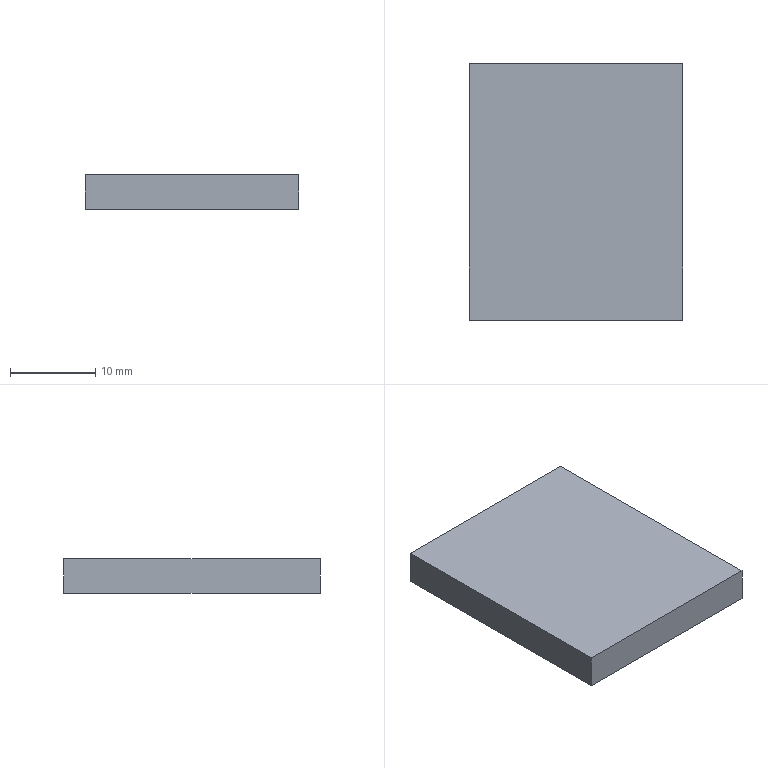Part | STEP file | Q7C0516 | 1 solid | 6 faces | box 25 x 30 x 4 mm | volume 3000 mm3 | plane 6
STEP:
#1=CARTESIAN_POINT('',(0.,0.,0.));
#2=DIRECTION('',(0.,0.,1.));
#3=DIRECTION('',(1.,0.,0.));
#4=AXIS2_PLACEMENT_3D('',#1,#2,#3);
#5=CARTESIAN_POINT('',(-25.,0.,0.));
#6=VERTEX_POINT('',#5);
#7=CARTESIAN_POINT('',(0.,0.,0.));
#8=VERTEX_POINT('',#7);
#9=CARTESIAN_POINT('',(-25.,0.,0.));
#10=DIRECTION('',(1.,0.,0.));
#11=VECTOR('',#10,1.);
#12=LINE('',#9,#11);
#13=CARTESIAN_POINT('',(-25.,0.,4.));
#14=DIRECTION('',(0.,1.,0.));
#15=DIRECTION('',(0.,0.,1.));
#16=AXIS2_PLACEMENT_3D('',#13,#14,#15);
#17=PLANE('',#16);
#18=CARTESIAN_POINT('',(-4.,0.));
#19=DIRECTION('',(0.,1.));
#20=VECTOR('',#19,1.);
#21=LINE('',#18,#20);
#22=(GEOMETRIC_REPRESENTATION_CONTEXT(2)PARAMETRIC_REPRESENTATION_CONTEXT()REPRESENTATION_CONTEXT('',''));
#23=DEFINITIONAL_REPRESENTATION('',(#21),#22);
#24=PCURVE('',#17,#23);
#25=CARTESIAN_POINT('',(0.,0.,0.));
#26=DIRECTION('',(0.,0.,1.));
#27=DIRECTION('',(1.,0.,0.));
#28=AXIS2_PLACEMENT_3D('',#25,#26,#27);
#29=PLANE('',#28);
#30=CARTESIAN_POINT('',(-25.,0.));
#31=DIRECTION('',(1.,0.));
#32=VECTOR('',#31,1.);
#33=LINE('',#30,#32);
#34=(GEOMETRIC_REPRESENTATION_CONTEXT(2)PARAMETRIC_REPRESENTATION_CONTEXT()REPRESENTATION_CONTEXT('',''));
#35=DEFINITIONAL_REPRESENTATION('',(#33),#34);
#36=PCURVE('',#29,#35);
#37=SURFACE_CURVE('',#12,(#24,#36),.PCURVE_S1.);
#38=EDGE_CURVE('',#6,#8,#37,.T.);
#39=ORIENTED_EDGE('',*,*,#38,.T.);
#40=CARTESIAN_POINT('',(0.,0.,4.));
#41=VERTEX_POINT('',#40);
#42=CARTESIAN_POINT('',(0.,0.,4.));
#43=DIRECTION('',(0.,0.,-1.));
#44=VECTOR('',#43,1.);
#45=LINE('',#42,#44);
#46=CARTESIAN_POINT('',(0.,25.));
#47=DIRECTION('',(-1.,0.));
#48=VECTOR('',#47,1.);
#49=LINE('',#46,#48);
#50=(GEOMETRIC_REPRESENTATION_CONTEXT(2)PARAMETRIC_REPRESENTATION_CONTEXT()REPRESENTATION_CONTEXT('',''));
#51=DEFINITIONAL_REPRESENTATION('',(#49),#50);
#52=PCURVE('',#17,#51);
#53=CARTESIAN_POINT('',(0.,0.,4.));
#54=DIRECTION('',(-1.,0.,0.));
#55=DIRECTION('',(0.,0.,1.));
#56=AXIS2_PLACEMENT_3D('',#53,#54,#55);
#57=PLANE('',#56);
#58=CARTESIAN_POINT('',(0.,0.));
#59=DIRECTION('',(-1.,0.));
#60=VECTOR('',#59,1.);
#61=LINE('',#58,#60);
#62=(GEOMETRIC_REPRESENTATION_CONTEXT(2)PARAMETRIC_REPRESENTATION_CONTEXT()REPRESENTATION_CONTEXT('',''));
#63=DEFINITIONAL_REPRESENTATION('',(#61),#62);
#64=PCURVE('',#57,#63);
#65=SURFACE_CURVE('',#45,(#52,#64),.PCURVE_S1.);
#66=EDGE_CURVE('',#41,#8,#65,.T.);
#67=ORIENTED_EDGE('',*,*,#66,.F.);
#68=CARTESIAN_POINT('',(-25.,0.,4.));
#69=VERTEX_POINT('',#68);
#70=CARTESIAN_POINT('',(-25.,0.,4.));
#71=DIRECTION('',(1.,0.,0.));
#72=VECTOR('',#71,1.);
#73=LINE('',#70,#72);
#74=CARTESIAN_POINT('',(0.,0.));
#75=DIRECTION('',(0.,1.));
#76=VECTOR('',#75,1.);
#77=LINE('',#74,#76);
#78=(GEOMETRIC_REPRESENTATION_CONTEXT(2)PARAMETRIC_REPRESENTATION_CONTEXT()REPRESENTATION_CONTEXT('',''));
#79=DEFINITIONAL_REPRESENTATION('',(#77),#78);
#80=PCURVE('',#17,#79);
#81=CARTESIAN_POINT('',(0.,0.,4.));
#82=DIRECTION('',(0.,0.,1.));
#83=DIRECTION('',(1.,0.,0.));
#84=AXIS2_PLACEMENT_3D('',#81,#82,#83);
#85=PLANE('',#84);
#86=CARTESIAN_POINT('',(-25.,0.));
#87=DIRECTION('',(1.,0.));
#88=VECTOR('',#87,1.);
#89=LINE('',#86,#88);
#90=(GEOMETRIC_REPRESENTATION_CONTEXT(2)PARAMETRIC_REPRESENTATION_CONTEXT()REPRESENTATION_CONTEXT('',''));
#91=DEFINITIONAL_REPRESENTATION('',(#89),#90);
#92=PCURVE('',#85,#91);
#93=SURFACE_CURVE('',#73,(#80,#92),.PCURVE_S1.);
#94=EDGE_CURVE('',#69,#41,#93,.T.);
#95=ORIENTED_EDGE('',*,*,#94,.F.);
#96=CARTESIAN_POINT('',(-25.,0.,4.));
#97=DIRECTION('',(0.,0.,-1.));
#98=VECTOR('',#97,1.);
#99=LINE('',#96,#98);
#100=CARTESIAN_POINT('',(0.,0.));
#101=DIRECTION('',(-1.,0.));
#102=VECTOR('',#101,1.);
#103=LINE('',#100,#102);
#104=(GEOMETRIC_REPRESENTATION_CONTEXT(2)PARAMETRIC_REPRESENTATION_CONTEXT()REPRESENTATION_CONTEXT('',''));
#105=DEFINITIONAL_REPRESENTATION('',(#103),#104);
#106=PCURVE('',#17,#105);
#107=CARTESIAN_POINT('',(-25.,0.,4.));
#108=DIRECTION('',(1.,0.,0.));
#109=DIRECTION('',(0.,0.,-1.));
#110=AXIS2_PLACEMENT_3D('',#107,#108,#109);
#111=PLANE('',#110);
#112=CARTESIAN_POINT('',(0.,0.));
#113=DIRECTION('',(1.,0.));
#114=VECTOR('',#113,1.);
#115=LINE('',#112,#114);
#116=(GEOMETRIC_REPRESENTATION_CONTEXT(2)PARAMETRIC_REPRESENTATION_CONTEXT()REPRESENTATION_CONTEXT('',''));
#117=DEFINITIONAL_REPRESENTATION('',(#115),#116);
#118=PCURVE('',#111,#117);
#119=SURFACE_CURVE('',#99,(#106,#118),.PCURVE_S1.);
#120=EDGE_CURVE('',#69,#6,#119,.T.);
#121=ORIENTED_EDGE('',*,*,#120,.T.);
#122=EDGE_LOOP('',(#39,#67,#95,#121));
#123=FACE_BOUND('',#122,.T.);
#124=ADVANCED_FACE('',(#123),#17,.F.);
#125=CARTESIAN_POINT('',(0.,30.,0.));
#126=VERTEX_POINT('',#125);
#127=CARTESIAN_POINT('',(0.,0.,0.));
#128=DIRECTION('',(0.,1.,0.));
#129=VECTOR('',#128,1.);
#130=LINE('',#127,#129);
#131=CARTESIAN_POINT('',(-4.,0.));
#132=DIRECTION('',(0.,1.));
#133=VECTOR('',#132,1.);
#134=LINE('',#131,#133);
#135=(GEOMETRIC_REPRESENTATION_CONTEXT(2)PARAMETRIC_REPRESENTATION_CONTEXT()REPRESENTATION_CONTEXT('',''));
#136=DEFINITIONAL_REPRESENTATION('',(#134),#135);
#137=PCURVE('',#57,#136);
#138=CARTESIAN_POINT('',(0.,0.));
#139=DIRECTION('',(0.,1.));
#140=VECTOR('',#139,1.);
#141=LINE('',#138,#140);
#142=(GEOMETRIC_REPRESENTATION_CONTEXT(2)PARAMETRIC_REPRESENTATION_CONTEXT()REPRESENTATION_CONTEXT('',''));
#143=DEFINITIONAL_REPRESENTATION('',(#141),#142);
#144=PCURVE('',#29,#143);
#145=SURFACE_CURVE('',#130,(#137,#144),.PCURVE_S1.);
#146=EDGE_CURVE('',#8,#126,#145,.T.);
#147=ORIENTED_EDGE('',*,*,#146,.T.);
#148=CARTESIAN_POINT('',(0.,30.,4.));
#149=VERTEX_POINT('',#148);
#150=CARTESIAN_POINT('',(0.,30.,4.));
#151=DIRECTION('',(0.,0.,-1.));
#152=VECTOR('',#151,1.);
#153=LINE('',#150,#152);
#154=CARTESIAN_POINT('',(0.,30.));
#155=DIRECTION('',(-1.,0.));
#156=VECTOR('',#155,1.);
#157=LINE('',#154,#156);
#158=(GEOMETRIC_REPRESENTATION_CONTEXT(2)PARAMETRIC_REPRESENTATION_CONTEXT()REPRESENTATION_CONTEXT('',''));
#159=DEFINITIONAL_REPRESENTATION('',(#157),#158);
#160=PCURVE('',#57,#159);
#161=CARTESIAN_POINT('',(-25.,30.,4.));
#162=DIRECTION('',(0.,-1.,0.));
#163=DIRECTION('',(0.,0.,-1.));
#164=AXIS2_PLACEMENT_3D('',#161,#162,#163);
#165=PLANE('',#164);
#166=CARTESIAN_POINT('',(0.,25.));
#167=DIRECTION('',(1.,0.));
#168=VECTOR('',#167,1.);
#169=LINE('',#166,#168);
#170=(GEOMETRIC_REPRESENTATION_CONTEXT(2)PARAMETRIC_REPRESENTATION_CONTEXT()REPRESENTATION_CONTEXT('',''));
#171=DEFINITIONAL_REPRESENTATION('',(#169),#170);
#172=PCURVE('',#165,#171);
#173=SURFACE_CURVE('',#153,(#160,#172),.PCURVE_S1.);
#174=EDGE_CURVE('',#149,#126,#173,.T.);
#175=ORIENTED_EDGE('',*,*,#174,.F.);
#176=CARTESIAN_POINT('',(0.,0.,4.));
#177=DIRECTION('',(0.,1.,0.));
#178=VECTOR('',#177,1.);
#179=LINE('',#176,#178);
#180=CARTESIAN_POINT('',(0.,0.));
#181=DIRECTION('',(0.,1.));
#182=VECTOR('',#181,1.);
#183=LINE('',#180,#182);
#184=(GEOMETRIC_REPRESENTATION_CONTEXT(2)PARAMETRIC_REPRESENTATION_CONTEXT()REPRESENTATION_CONTEXT('',''));
#185=DEFINITIONAL_REPRESENTATION('',(#183),#184);
#186=PCURVE('',#57,#185);
#187=CARTESIAN_POINT('',(0.,0.));
#188=DIRECTION('',(0.,1.));
#189=VECTOR('',#188,1.);
#190=LINE('',#187,#189);
#191=(GEOMETRIC_REPRESENTATION_CONTEXT(2)PARAMETRIC_REPRESENTATION_CONTEXT()REPRESENTATION_CONTEXT('',''));
#192=DEFINITIONAL_REPRESENTATION('',(#190),#191);
#193=PCURVE('',#85,#192);
#194=SURFACE_CURVE('',#179,(#186,#193),.PCURVE_S1.);
#195=EDGE_CURVE('',#41,#149,#194,.T.);
#196=ORIENTED_EDGE('',*,*,#195,.F.);
#197=ORIENTED_EDGE('',*,*,#66,.T.);
#198=EDGE_LOOP('',(#147,#175,#196,#197));
#199=FACE_BOUND('',#198,.T.);
#200=ADVANCED_FACE('',(#199),#57,.F.);
#201=CARTESIAN_POINT('',(-25.,30.,0.));
#202=VERTEX_POINT('',#201);
#203=CARTESIAN_POINT('',(-25.,30.,0.));
#204=DIRECTION('',(-1.,0.,0.));
#205=VECTOR('',#204,1.);
#206=LINE('',#203,#205);
#207=CARTESIAN_POINT('',(4.,0.));
#208=DIRECTION('',(0.,-1.));
#209=VECTOR('',#208,1.);
#210=LINE('',#207,#209);
#211=(GEOMETRIC_REPRESENTATION_CONTEXT(2)PARAMETRIC_REPRESENTATION_CONTEXT()REPRESENTATION_CONTEXT('',''));
#212=DEFINITIONAL_REPRESENTATION('',(#210),#211);
#213=PCURVE('',#165,#212);
#214=CARTESIAN_POINT('',(-25.,30.));
#215=DIRECTION('',(-1.,0.));
#216=VECTOR('',#215,1.);
#217=LINE('',#214,#216);
#218=(GEOMETRIC_REPRESENTATION_CONTEXT(2)PARAMETRIC_REPRESENTATION_CONTEXT()REPRESENTATION_CONTEXT('',''));
#219=DEFINITIONAL_REPRESENTATION('',(#217),#218);
#220=PCURVE('',#29,#219);
#221=SURFACE_CURVE('',#206,(#213,#220),.PCURVE_S1.);
#222=EDGE_CURVE('',#126,#202,#221,.T.);
#223=ORIENTED_EDGE('',*,*,#222,.T.);
#224=CARTESIAN_POINT('',(-25.,30.,4.));
#225=VERTEX_POINT('',#224);
#226=CARTESIAN_POINT('',(-25.,30.,4.));
#227=DIRECTION('',(0.,0.,-1.));
#228=VECTOR('',#227,1.);
#229=LINE('',#226,#228);
#230=CARTESIAN_POINT('',(0.,0.));
#231=DIRECTION('',(1.,0.));
#232=VECTOR('',#231,1.);
#233=LINE('',#230,#232);
#234=(GEOMETRIC_REPRESENTATION_CONTEXT(2)PARAMETRIC_REPRESENTATION_CONTEXT()REPRESENTATION_CONTEXT('',''));
#235=DEFINITIONAL_REPRESENTATION('',(#233),#234);
#236=PCURVE('',#165,#235);
#237=CARTESIAN_POINT('',(0.,30.));
#238=DIRECTION('',(1.,0.));
#239=VECTOR('',#238,1.);
#240=LINE('',#237,#239);
#241=(GEOMETRIC_REPRESENTATION_CONTEXT(2)PARAMETRIC_REPRESENTATION_CONTEXT()REPRESENTATION_CONTEXT('',''));
#242=DEFINITIONAL_REPRESENTATION('',(#240),#241);
#243=PCURVE('',#111,#242);
#244=SURFACE_CURVE('',#229,(#236,#243),.PCURVE_S1.);
#245=EDGE_CURVE('',#225,#202,#244,.T.);
#246=ORIENTED_EDGE('',*,*,#245,.F.);
#247=CARTESIAN_POINT('',(-25.,30.,4.));
#248=DIRECTION('',(-1.,0.,0.));
#249=VECTOR('',#248,1.);
#250=LINE('',#247,#249);
#251=CARTESIAN_POINT('',(0.,0.));
#252=DIRECTION('',(0.,-1.));
#253=VECTOR('',#252,1.);
#254=LINE('',#251,#253);
#255=(GEOMETRIC_REPRESENTATION_CONTEXT(2)PARAMETRIC_REPRESENTATION_CONTEXT()REPRESENTATION_CONTEXT('',''));
#256=DEFINITIONAL_REPRESENTATION('',(#254),#255);
#257=PCURVE('',#165,#256);
#258=CARTESIAN_POINT('',(-25.,30.));
#259=DIRECTION('',(-1.,0.));
#260=VECTOR('',#259,1.);
#261=LINE('',#258,#260);
#262=(GEOMETRIC_REPRESENTATION_CONTEXT(2)PARAMETRIC_REPRESENTATION_CONTEXT()REPRESENTATION_CONTEXT('',''));
#263=DEFINITIONAL_REPRESENTATION('',(#261),#262);
#264=PCURVE('',#85,#263);
#265=SURFACE_CURVE('',#250,(#257,#264),.PCURVE_S1.);
#266=EDGE_CURVE('',#149,#225,#265,.T.);
#267=ORIENTED_EDGE('',*,*,#266,.F.);
#268=ORIENTED_EDGE('',*,*,#174,.T.);
#269=EDGE_LOOP('',(#223,#246,#267,#268));
#270=FACE_BOUND('',#269,.T.);
#271=ADVANCED_FACE('',(#270),#165,.F.);
#272=CARTESIAN_POINT('',(-25.,0.,0.));
#273=DIRECTION('',(0.,-1.,0.));
#274=VECTOR('',#273,1.);
#275=LINE('',#272,#274);
#276=CARTESIAN_POINT('',(4.,0.));
#277=DIRECTION('',(0.,-1.));
#278=VECTOR('',#277,1.);
#279=LINE('',#276,#278);
#280=(GEOMETRIC_REPRESENTATION_CONTEXT(2)PARAMETRIC_REPRESENTATION_CONTEXT()REPRESENTATION_CONTEXT('',''));
#281=DEFINITIONAL_REPRESENTATION('',(#279),#280);
#282=PCURVE('',#111,#281);
#283=CARTESIAN_POINT('',(-25.,0.));
#284=DIRECTION('',(0.,-1.));
#285=VECTOR('',#284,1.);
#286=LINE('',#283,#285);
#287=(GEOMETRIC_REPRESENTATION_CONTEXT(2)PARAMETRIC_REPRESENTATION_CONTEXT()REPRESENTATION_CONTEXT('',''));
#288=DEFINITIONAL_REPRESENTATION('',(#286),#287);
#289=PCURVE('',#29,#288);
#290=SURFACE_CURVE('',#275,(#282,#289),.PCURVE_S1.);
#291=EDGE_CURVE('',#202,#6,#290,.T.);
#292=ORIENTED_EDGE('',*,*,#291,.T.);
#293=ORIENTED_EDGE('',*,*,#120,.F.);
#294=CARTESIAN_POINT('',(-25.,0.,4.));
#295=DIRECTION('',(0.,-1.,0.));
#296=VECTOR('',#295,1.);
#297=LINE('',#294,#296);
#298=CARTESIAN_POINT('',(0.,0.));
#299=DIRECTION('',(0.,-1.));
#300=VECTOR('',#299,1.);
#301=LINE('',#298,#300);
#302=(GEOMETRIC_REPRESENTATION_CONTEXT(2)PARAMETRIC_REPRESENTATION_CONTEXT()REPRESENTATION_CONTEXT('',''));
#303=DEFINITIONAL_REPRESENTATION('',(#301),#302);
#304=PCURVE('',#111,#303);
#305=CARTESIAN_POINT('',(-25.,0.));
#306=DIRECTION('',(0.,-1.));
#307=VECTOR('',#306,1.);
#308=LINE('',#305,#307);
#309=(GEOMETRIC_REPRESENTATION_CONTEXT(2)PARAMETRIC_REPRESENTATION_CONTEXT()REPRESENTATION_CONTEXT('',''));
#310=DEFINITIONAL_REPRESENTATION('',(#308),#309);
#311=PCURVE('',#85,#310);
#312=SURFACE_CURVE('',#297,(#304,#311),.PCURVE_S1.);
#313=EDGE_CURVE('',#225,#69,#312,.T.);
#314=ORIENTED_EDGE('',*,*,#313,.F.);
#315=ORIENTED_EDGE('',*,*,#245,.T.);
#316=EDGE_LOOP('',(#292,#293,#314,#315));
#317=FACE_BOUND('',#316,.T.);
#318=ADVANCED_FACE('',(#317),#111,.F.);
#319=ORIENTED_EDGE('',*,*,#94,.T.);
#320=ORIENTED_EDGE('',*,*,#195,.T.);
#321=ORIENTED_EDGE('',*,*,#266,.T.);
#322=ORIENTED_EDGE('',*,*,#313,.T.);
#323=EDGE_LOOP('',(#319,#320,#321,#322));
#324=FACE_BOUND('',#323,.T.);
#325=ADVANCED_FACE('',(#324),#85,.T.);
#326=ORIENTED_EDGE('',*,*,#38,.F.);
#327=ORIENTED_EDGE('',*,*,#291,.F.);
#328=ORIENTED_EDGE('',*,*,#222,.F.);
#329=ORIENTED_EDGE('',*,*,#146,.F.);
#330=EDGE_LOOP('',(#326,#327,#328,#329));
#331=FACE_BOUND('',#330,.T.);
#332=ADVANCED_FACE('',(#331),#29,.F.);
#333=CLOSED_SHELL('',(#124,#200,#271,#318,#325,#332));
#334=MANIFOLD_SOLID_BREP('',#333);
#335=(LENGTH_UNIT()NAMED_UNIT(*)SI_UNIT(.MILLI.,.METRE.));
#336=UNCERTAINTY_MEASURE_WITH_UNIT(LENGTH_MEASURE(0.0000001),#335,'','');
#337=(NAMED_UNIT(*)PLANE_ANGLE_UNIT()SI_UNIT($,.RADIAN.));
#338=(NAMED_UNIT(*)SI_UNIT($,.STERADIAN.)SOLID_ANGLE_UNIT());
#339=(GEOMETRIC_REPRESENTATION_CONTEXT(3)GLOBAL_UNCERTAINTY_ASSIGNED_CONTEXT((#336))GLOBAL_UNIT_ASSIGNED_CONTEXT((#335,#337,#338))REPRESENTATION_CONTEXT('',''));
#340=ADVANCED_BREP_SHAPE_REPRESENTATION('',(#4,#334),#339);